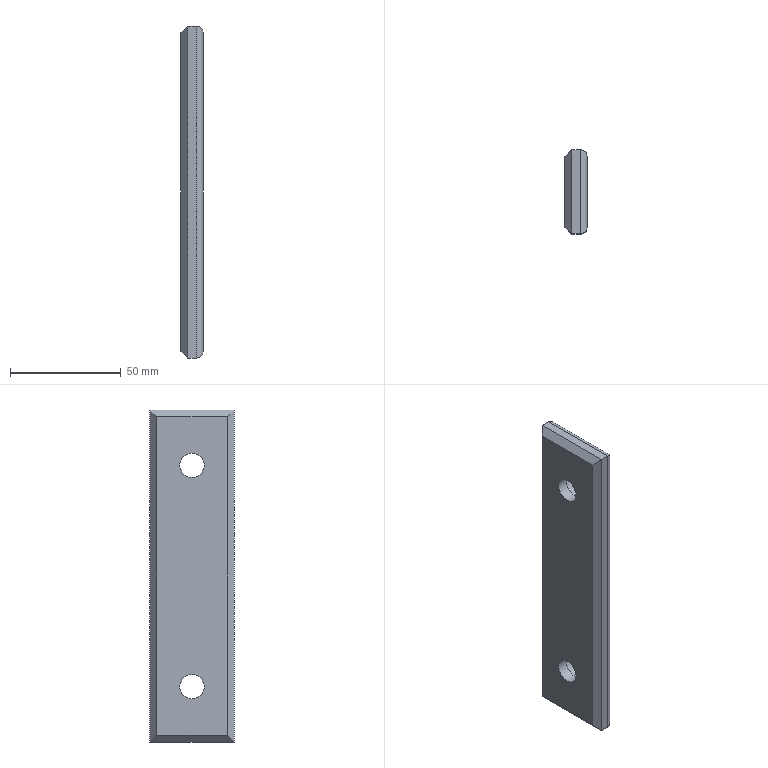Part | NX | features solid 2 | 1 solid | 20 faces | box 10 x 38 x 150 mm | volume 51273 mm3 | plane 12 | cylinder 8 | commonest cylinder face diameters 6 x4 11 x2 17.5 x2
STEP:
#1=CARTESIAN_POINT('',(163.,430.,45.));
#2=VERTEX_POINT('',#1);
#3=CARTESIAN_POINT('',(167.,430.,45.));
#4=VERTEX_POINT('',#3);
#5=CARTESIAN_POINT('',(160.,430.,45.));
#6=DIRECTION('',(1.,0.,0.));
#7=VECTOR('',#6,1000.);
#8=LINE('',#5,#7);
#9=EDGE_CURVE('',#2,#4,#8,.T.);
#10=ORIENTED_EDGE('',*,*,#9,.T.);
#11=CARTESIAN_POINT('',(167.,392.,45.));
#12=VERTEX_POINT('',#11);
#13=CARTESIAN_POINT('',(167.,392.,45.));
#14=DIRECTION('',(0.,1.,0.));
#15=VECTOR('',#14,1000.);
#16=LINE('',#13,#15);
#17=EDGE_CURVE('',#12,#4,#16,.T.);
#18=ORIENTED_EDGE('',*,*,#17,.F.);
#19=CARTESIAN_POINT('',(163.,392.,45.));
#20=VERTEX_POINT('',#19);
#21=CARTESIAN_POINT('',(160.,392.,45.));
#22=DIRECTION('',(1.,0.,0.));
#23=VECTOR('',#22,1000.);
#24=LINE('',#21,#23);
#25=EDGE_CURVE('',#20,#12,#24,.T.);
#26=ORIENTED_EDGE('',*,*,#25,.F.);
#27=CARTESIAN_POINT('',(163.,392.,45.));
#28=DIRECTION('',(0.,-1.,0.));
#29=VECTOR('',#28,1000.);
#30=LINE('',#27,#29);
#31=EDGE_CURVE('',#2,#20,#30,.T.);
#32=ORIENTED_EDGE('',*,*,#31,.F.);
#33=EDGE_LOOP('',(#10,#18,#26,#32));
#34=FACE_BOUND('',#33,.T.);
#35=CARTESIAN_POINT('',(160.,392.,45.));
#36=DIRECTION('',(0.,0.,1.));
#37=DIRECTION('',(1.,0.,0.));
#38=AXIS2_PLACEMENT_3D('',#35,#36,#37);
#39=PLANE('',#38);
#40=ADVANCED_FACE('',(#34),#39,.F.);
#41=CARTESIAN_POINT('',(163.,430.,195.));
#42=VERTEX_POINT('',#41);
#43=CARTESIAN_POINT('',(167.,430.,195.));
#44=VERTEX_POINT('',#43);
#45=CARTESIAN_POINT('',(160.,430.,195.));
#46=DIRECTION('',(1.,0.,0.));
#47=VECTOR('',#46,1000.);
#48=LINE('',#45,#47);
#49=EDGE_CURVE('',#42,#44,#48,.T.);
#50=ORIENTED_EDGE('',*,*,#49,.T.);
#51=CARTESIAN_POINT('',(167.,430.,45.));
#52=DIRECTION('',(0.,0.,1.));
#53=VECTOR('',#52,1000.);
#54=LINE('',#51,#53);
#55=EDGE_CURVE('',#4,#44,#54,.T.);
#56=ORIENTED_EDGE('',*,*,#55,.F.);
#57=ORIENTED_EDGE('',*,*,#9,.F.);
#58=CARTESIAN_POINT('',(163.,430.,45.));
#59=DIRECTION('',(0.,0.,-1.));
#60=VECTOR('',#59,1000.);
#61=LINE('',#58,#60);
#62=EDGE_CURVE('',#42,#2,#61,.T.);
#63=ORIENTED_EDGE('',*,*,#62,.F.);
#64=EDGE_LOOP('',(#50,#56,#57,#63));
#65=FACE_BOUND('',#64,.T.);
#66=CARTESIAN_POINT('',(160.,430.,45.));
#67=DIRECTION('',(0.,-1.,0.));
#68=DIRECTION('',(-1.,0.,0.));
#69=AXIS2_PLACEMENT_3D('',#66,#67,#68);
#70=PLANE('',#69);
#71=ADVANCED_FACE('',(#65),#70,.F.);
#72=CARTESIAN_POINT('',(163.,392.,195.));
#73=VERTEX_POINT('',#72);
#74=CARTESIAN_POINT('',(167.,392.,195.));
#75=VERTEX_POINT('',#74);
#76=CARTESIAN_POINT('',(160.,392.,195.));
#77=DIRECTION('',(1.,0.,0.));
#78=VECTOR('',#77,1000.);
#79=LINE('',#76,#78);
#80=EDGE_CURVE('',#73,#75,#79,.T.);
#81=ORIENTED_EDGE('',*,*,#80,.T.);
#82=CARTESIAN_POINT('',(167.,430.,195.));
#83=DIRECTION('',(0.,-1.,0.));
#84=VECTOR('',#83,1000.);
#85=LINE('',#82,#84);
#86=EDGE_CURVE('',#44,#75,#85,.T.);
#87=ORIENTED_EDGE('',*,*,#86,.F.);
#88=ORIENTED_EDGE('',*,*,#49,.F.);
#89=CARTESIAN_POINT('',(163.,430.,195.));
#90=DIRECTION('',(0.,1.,0.));
#91=VECTOR('',#90,1000.);
#92=LINE('',#89,#91);
#93=EDGE_CURVE('',#73,#42,#92,.T.);
#94=ORIENTED_EDGE('',*,*,#93,.F.);
#95=EDGE_LOOP('',(#81,#87,#88,#94));
#96=FACE_BOUND('',#95,.T.);
#97=CARTESIAN_POINT('',(160.,430.,195.));
#98=DIRECTION('',(0.,0.,-1.));
#99=DIRECTION('',(0.,1.,0.));
#100=AXIS2_PLACEMENT_3D('',#97,#98,#99);
#101=PLANE('',#100);
#102=ADVANCED_FACE('',(#96),#101,.F.);
#103=ORIENTED_EDGE('',*,*,#25,.T.);
#104=CARTESIAN_POINT('',(167.,392.,145.));
#105=DIRECTION('',(0.,0.,-1.));
#106=VECTOR('',#105,1000.);
#107=LINE('',#104,#106);
#108=EDGE_CURVE('',#75,#12,#107,.T.);
#109=ORIENTED_EDGE('',*,*,#108,.F.);
#110=ORIENTED_EDGE('',*,*,#80,.F.);
#111=CARTESIAN_POINT('',(163.,392.,145.));
#112=DIRECTION('',(0.,0.,1.));
#113=VECTOR('',#112,1000.);
#114=LINE('',#111,#113);
#115=EDGE_CURVE('',#20,#73,#114,.T.);
#116=ORIENTED_EDGE('',*,*,#115,.F.);
#117=EDGE_LOOP('',(#103,#109,#110,#116));
#118=FACE_BOUND('',#117,.T.);
#119=CARTESIAN_POINT('',(160.,392.,145.));
#120=DIRECTION('',(0.,1.,0.));
#121=DIRECTION('',(0.,0.,1.));
#122=AXIS2_PLACEMENT_3D('',#119,#120,#121);
#123=PLANE('',#122);
#124=ADVANCED_FACE('',(#118),#123,.F.);
#125=CARTESIAN_POINT('',(160.,427.,48.));
#126=VERTEX_POINT('',#125);
#127=CARTESIAN_POINT('',(160.,427.,192.));
#128=VERTEX_POINT('',#127);
#129=CARTESIAN_POINT('',(160.,427.,145.));
#130=DIRECTION('',(0.,0.,1.));
#131=VECTOR('',#130,1000.);
#132=LINE('',#129,#131);
#133=EDGE_CURVE('',#126,#128,#132,.T.);
#134=ORIENTED_EDGE('',*,*,#133,.F.);
#135=CARTESIAN_POINT('',(160.,395.,48.));
#136=VERTEX_POINT('',#135);
#137=CARTESIAN_POINT('',(160.,430.,48.));
#138=DIRECTION('',(0.,1.,0.));
#139=VECTOR('',#138,1000.);
#140=LINE('',#137,#139);
#141=EDGE_CURVE('',#136,#126,#140,.T.);
#142=ORIENTED_EDGE('',*,*,#141,.F.);
#143=CARTESIAN_POINT('',(160.,395.,192.));
#144=VERTEX_POINT('',#143);
#145=CARTESIAN_POINT('',(160.,395.,45.));
#146=DIRECTION('',(0.,0.,-1.));
#147=VECTOR('',#146,1000.);
#148=LINE('',#145,#147);
#149=EDGE_CURVE('',#144,#136,#148,.T.);
#150=ORIENTED_EDGE('',*,*,#149,.F.);
#151=CARTESIAN_POINT('',(160.,392.,192.));
#152=DIRECTION('',(0.,-1.,0.));
#153=VECTOR('',#152,1000.);
#154=LINE('',#151,#153);
#155=EDGE_CURVE('',#128,#144,#154,.T.);
#156=ORIENTED_EDGE('',*,*,#155,.F.);
#157=EDGE_LOOP('',(#134,#142,#150,#156));
#158=FACE_BOUND('',#157,.T.);
#159=CARTESIAN_POINT('',(160.,411.,175.5));
#160=VERTEX_POINT('',#159);
#161=CARTESIAN_POINT('',(160.,411.,170.));
#162=DIRECTION('',(1.,0.,0.));
#163=DIRECTION('',(0.,0.,1.));
#164=AXIS2_PLACEMENT_3D('',#161,#162,#163);
#165=CIRCLE('',#164,5.5);
#166=EDGE_CURVE('',#160,#160,#165,.T.);
#167=ORIENTED_EDGE('',*,*,#166,.T.);
#168=EDGE_LOOP('',(#167));
#169=FACE_BOUND('',#168,.T.);
#170=CARTESIAN_POINT('',(160.,411.,75.5));
#171=VERTEX_POINT('',#170);
#172=CARTESIAN_POINT('',(160.,411.,70.));
#173=DIRECTION('',(1.,0.,0.));
#174=DIRECTION('',(0.,0.,1.));
#175=AXIS2_PLACEMENT_3D('',#172,#173,#174);
#176=CIRCLE('',#175,5.5);
#177=EDGE_CURVE('',#171,#171,#176,.T.);
#178=ORIENTED_EDGE('',*,*,#177,.T.);
#179=EDGE_LOOP('',(#178));
#180=FACE_BOUND('',#179,.T.);
#181=CARTESIAN_POINT('',(160.,430.,45.));
#182=DIRECTION('',(-1.,0.,0.));
#183=DIRECTION('',(0.,0.,1.));
#184=AXIS2_PLACEMENT_3D('',#181,#182,#183);
#185=PLANE('',#184);
#186=ADVANCED_FACE('',(#158,#169,#180),#185,.T.);
#187=CARTESIAN_POINT('',(170.,427.,48.));
#188=VERTEX_POINT('',#187);
#189=CARTESIAN_POINT('',(170.,395.,48.));
#190=VERTEX_POINT('',#189);
#191=CARTESIAN_POINT('',(170.,430.,48.));
#192=DIRECTION('',(0.,1.,0.));
#193=VECTOR('',#192,1000.);
#194=LINE('',#191,#193);
#195=EDGE_CURVE('',#188,#190,#194,.F.);
#196=ORIENTED_EDGE('',*,*,#195,.F.);
#197=CARTESIAN_POINT('',(170.,427.,192.));
#198=VERTEX_POINT('',#197);
#199=CARTESIAN_POINT('',(170.,427.,45.));
#200=DIRECTION('',(0.,0.,1.));
#201=VECTOR('',#200,1000.);
#202=LINE('',#199,#201);
#203=EDGE_CURVE('',#198,#188,#202,.F.);
#204=ORIENTED_EDGE('',*,*,#203,.F.);
#205=CARTESIAN_POINT('',(170.,395.,192.));
#206=VERTEX_POINT('',#205);
#207=CARTESIAN_POINT('',(170.,430.,192.));
#208=DIRECTION('',(0.,-1.,0.));
#209=VECTOR('',#208,1000.);
#210=LINE('',#207,#209);
#211=EDGE_CURVE('',#206,#198,#210,.F.);
#212=ORIENTED_EDGE('',*,*,#211,.F.);
#213=CARTESIAN_POINT('',(170.,395.,45.));
#214=DIRECTION('',(0.,0.,-1.));
#215=VECTOR('',#214,1000.);
#216=LINE('',#213,#215);
#217=EDGE_CURVE('',#190,#206,#216,.F.);
#218=ORIENTED_EDGE('',*,*,#217,.F.);
#219=EDGE_LOOP('',(#196,#204,#212,#218));
#220=FACE_BOUND('',#219,.T.);
#221=CARTESIAN_POINT('',(170.,411.,178.75));
#222=VERTEX_POINT('',#221);
#223=CARTESIAN_POINT('',(170.,411.,170.));
#224=DIRECTION('',(1.,0.,0.));
#225=DIRECTION('',(0.,0.,1.));
#226=AXIS2_PLACEMENT_3D('',#223,#224,#225);
#227=CIRCLE('',#226,8.75);
#228=EDGE_CURVE('',#222,#222,#227,.T.);
#229=ORIENTED_EDGE('',*,*,#228,.F.);
#230=EDGE_LOOP('',(#229));
#231=FACE_BOUND('',#230,.T.);
#232=CARTESIAN_POINT('',(170.,411.,78.75));
#233=VERTEX_POINT('',#232);
#234=CARTESIAN_POINT('',(170.,411.,70.));
#235=DIRECTION('',(1.,0.,0.));
#236=DIRECTION('',(0.,0.,1.));
#237=AXIS2_PLACEMENT_3D('',#234,#235,#236);
#238=CIRCLE('',#237,8.75);
#239=EDGE_CURVE('',#233,#233,#238,.T.);
#240=ORIENTED_EDGE('',*,*,#239,.F.);
#241=EDGE_LOOP('',(#240));
#242=FACE_BOUND('',#241,.T.);
#243=CARTESIAN_POINT('',(170.,430.,45.));
#244=DIRECTION('',(-1.,0.,0.));
#245=DIRECTION('',(0.,0.,1.));
#246=AXIS2_PLACEMENT_3D('',#243,#244,#245);
#247=PLANE('',#246);
#248=ADVANCED_FACE('',(#220,#231,#242),#247,.F.);
#249=ORIENTED_EDGE('',*,*,#177,.F.);
#250=EDGE_LOOP('',(#249));
#251=FACE_BOUND('',#250,.T.);
#252=CARTESIAN_POINT('',(165.,411.,64.5));
#253=VERTEX_POINT('',#252);
#254=CARTESIAN_POINT('',(165.,411.,70.));
#255=DIRECTION('',(1.,0.,0.));
#256=DIRECTION('',(0.,0.,-1.));
#257=AXIS2_PLACEMENT_3D('',#254,#255,#256);
#258=CIRCLE('',#257,5.5);
#259=EDGE_CURVE('',#253,#253,#258,.T.);
#260=ORIENTED_EDGE('',*,*,#259,.T.);
#261=EDGE_LOOP('',(#260));
#262=FACE_BOUND('',#261,.T.);
#263=CARTESIAN_POINT('',(130.,411.,70.));
#264=DIRECTION('',(-1.,0.,0.));
#265=DIRECTION('',(0.,0.,1.));
#266=AXIS2_PLACEMENT_3D('',#263,#264,#265);
#267=CYLINDRICAL_SURFACE('',#266,5.5);
#268=ADVANCED_FACE('',(#251,#262),#267,.F.);
#269=ORIENTED_EDGE('',*,*,#259,.F.);
#270=EDGE_LOOP('',(#269));
#271=FACE_BOUND('',#270,.T.);
#272=CARTESIAN_POINT('',(165.,411.,61.25));
#273=VERTEX_POINT('',#272);
#274=CARTESIAN_POINT('',(165.,411.,70.));
#275=DIRECTION('',(1.,0.,0.));
#276=DIRECTION('',(0.,0.,-1.));
#277=AXIS2_PLACEMENT_3D('',#274,#275,#276);
#278=CIRCLE('',#277,8.75);
#279=EDGE_CURVE('',#273,#273,#278,.T.);
#280=ORIENTED_EDGE('',*,*,#279,.T.);
#281=EDGE_LOOP('',(#280));
#282=FACE_BOUND('',#281,.T.);
#283=CARTESIAN_POINT('',(165.,411.,70.));
#284=DIRECTION('',(-1.,0.,0.));
#285=DIRECTION('',(0.,0.,1.));
#286=AXIS2_PLACEMENT_3D('',#283,#284,#285);
#287=PLANE('',#286);
#288=ADVANCED_FACE('',(#271,#282),#287,.F.);
#289=ORIENTED_EDGE('',*,*,#279,.F.);
#290=EDGE_LOOP('',(#289));
#291=FACE_BOUND('',#290,.T.);
#292=ORIENTED_EDGE('',*,*,#239,.T.);
#293=EDGE_LOOP('',(#292));
#294=FACE_BOUND('',#293,.T.);
#295=CARTESIAN_POINT('',(180.,411.,70.));
#296=DIRECTION('',(-1.,0.,0.));
#297=DIRECTION('',(0.,0.,1.));
#298=AXIS2_PLACEMENT_3D('',#295,#296,#297);
#299=CYLINDRICAL_SURFACE('',#298,8.75);
#300=ADVANCED_FACE('',(#291,#294),#299,.F.);
#301=ORIENTED_EDGE('',*,*,#166,.F.);
#302=EDGE_LOOP('',(#301));
#303=FACE_BOUND('',#302,.T.);
#304=CARTESIAN_POINT('',(165.,411.,164.5));
#305=VERTEX_POINT('',#304);
#306=CARTESIAN_POINT('',(165.,411.,170.));
#307=DIRECTION('',(1.,0.,0.));
#308=DIRECTION('',(0.,0.,-1.));
#309=AXIS2_PLACEMENT_3D('',#306,#307,#308);
#310=CIRCLE('',#309,5.5);
#311=EDGE_CURVE('',#305,#305,#310,.T.);
#312=ORIENTED_EDGE('',*,*,#311,.T.);
#313=EDGE_LOOP('',(#312));
#314=FACE_BOUND('',#313,.T.);
#315=CARTESIAN_POINT('',(130.,411.,170.));
#316=DIRECTION('',(-1.,0.,0.));
#317=DIRECTION('',(0.,0.,1.));
#318=AXIS2_PLACEMENT_3D('',#315,#316,#317);
#319=CYLINDRICAL_SURFACE('',#318,5.5);
#320=ADVANCED_FACE('',(#303,#314),#319,.F.);
#321=ORIENTED_EDGE('',*,*,#311,.F.);
#322=EDGE_LOOP('',(#321));
#323=FACE_BOUND('',#322,.T.);
#324=CARTESIAN_POINT('',(165.,411.,161.25));
#325=VERTEX_POINT('',#324);
#326=CARTESIAN_POINT('',(165.,411.,170.));
#327=DIRECTION('',(1.,0.,0.));
#328=DIRECTION('',(0.,0.,-1.));
#329=AXIS2_PLACEMENT_3D('',#326,#327,#328);
#330=CIRCLE('',#329,8.75);
#331=EDGE_CURVE('',#325,#325,#330,.T.);
#332=ORIENTED_EDGE('',*,*,#331,.T.);
#333=EDGE_LOOP('',(#332));
#334=FACE_BOUND('',#333,.T.);
#335=CARTESIAN_POINT('',(165.,411.,120.));
#336=DIRECTION('',(-1.,0.,0.));
#337=DIRECTION('',(0.,0.,1.));
#338=AXIS2_PLACEMENT_3D('',#335,#336,#337);
#339=PLANE('',#338);
#340=ADVANCED_FACE('',(#323,#334),#339,.F.);
#341=ORIENTED_EDGE('',*,*,#331,.F.);
#342=EDGE_LOOP('',(#341));
#343=FACE_BOUND('',#342,.T.);
#344=ORIENTED_EDGE('',*,*,#228,.T.);
#345=EDGE_LOOP('',(#344));
#346=FACE_BOUND('',#345,.T.);
#347=CARTESIAN_POINT('',(180.,411.,170.));
#348=DIRECTION('',(-1.,0.,0.));
#349=DIRECTION('',(0.,0.,1.));
#350=AXIS2_PLACEMENT_3D('',#347,#348,#349);
#351=CYLINDRICAL_SURFACE('',#350,8.75);
#352=ADVANCED_FACE('',(#343,#346),#351,.F.);
#353=CARTESIAN_POINT('',(167.,427.,48.));
#354=DIRECTION('',(0.,-0.7071,-0.7071));
#355=DIRECTION('',(0.,0.7071,-0.7071));
#356=AXIS2_PLACEMENT_3D('',#353,#354,#355);
#357=ELLIPSE('',#356,4.243,3.);
#358=EDGE_CURVE('',#188,#4,#357,.F.);
#359=ORIENTED_EDGE('',*,*,#358,.T.);
#360=ORIENTED_EDGE('',*,*,#55,.T.);
#361=CARTESIAN_POINT('',(167.,427.,192.));
#362=DIRECTION('',(0.,0.7071,-0.7071));
#363=DIRECTION('',(0.,0.7071,0.7071));
#364=AXIS2_PLACEMENT_3D('',#361,#362,#363);
#365=ELLIPSE('',#364,4.243,3.);
#366=EDGE_CURVE('',#44,#198,#365,.T.);
#367=ORIENTED_EDGE('',*,*,#366,.T.);
#368=ORIENTED_EDGE('',*,*,#203,.T.);
#369=EDGE_LOOP('',(#359,#360,#367,#368));
#370=FACE_BOUND('',#369,.T.);
#371=CARTESIAN_POINT('',(167.,427.,45.));
#372=DIRECTION('',(0.,0.,1.));
#373=DIRECTION('',(1.,0.,0.));
#374=AXIS2_PLACEMENT_3D('',#371,#372,#373);
#375=CYLINDRICAL_SURFACE('',#374,3.);
#376=ADVANCED_FACE('',(#370),#375,.T.);
#377=ORIENTED_EDGE('',*,*,#366,.F.);
#378=ORIENTED_EDGE('',*,*,#86,.T.);
#379=CARTESIAN_POINT('',(167.,395.,192.));
#380=DIRECTION('',(0.,0.7071,0.7071));
#381=DIRECTION('',(0.,-0.7071,0.7071));
#382=AXIS2_PLACEMENT_3D('',#379,#380,#381);
#383=ELLIPSE('',#382,4.243,3.);
#384=EDGE_CURVE('',#75,#206,#383,.T.);
#385=ORIENTED_EDGE('',*,*,#384,.T.);
#386=ORIENTED_EDGE('',*,*,#211,.T.);
#387=EDGE_LOOP('',(#377,#378,#385,#386));
#388=FACE_BOUND('',#387,.T.);
#389=CARTESIAN_POINT('',(167.,430.,192.));
#390=DIRECTION('',(0.,-1.,0.));
#391=DIRECTION('',(0.,0.,-1.));
#392=AXIS2_PLACEMENT_3D('',#389,#390,#391);
#393=CYLINDRICAL_SURFACE('',#392,3.);
#394=ADVANCED_FACE('',(#388),#393,.T.);
#395=ORIENTED_EDGE('',*,*,#358,.F.);
#396=ORIENTED_EDGE('',*,*,#195,.T.);
#397=CARTESIAN_POINT('',(167.,395.,48.));
#398=DIRECTION('',(0.,-0.7071,0.7071));
#399=DIRECTION('',(0.,0.7071,0.7071));
#400=AXIS2_PLACEMENT_3D('',#397,#398,#399);
#401=ELLIPSE('',#400,4.243,3.);
#402=EDGE_CURVE('',#190,#12,#401,.F.);
#403=ORIENTED_EDGE('',*,*,#402,.T.);
#404=ORIENTED_EDGE('',*,*,#17,.T.);
#405=EDGE_LOOP('',(#395,#396,#403,#404));
#406=FACE_BOUND('',#405,.T.);
#407=CARTESIAN_POINT('',(167.,392.,48.));
#408=DIRECTION('',(0.,1.,0.));
#409=DIRECTION('',(1.,0.,0.));
#410=AXIS2_PLACEMENT_3D('',#407,#408,#409);
#411=CYLINDRICAL_SURFACE('',#410,3.);
#412=ADVANCED_FACE('',(#406),#411,.T.);
#413=ORIENTED_EDGE('',*,*,#384,.F.);
#414=ORIENTED_EDGE('',*,*,#108,.T.);
#415=ORIENTED_EDGE('',*,*,#402,.F.);
#416=ORIENTED_EDGE('',*,*,#217,.T.);
#417=EDGE_LOOP('',(#413,#414,#415,#416));
#418=FACE_BOUND('',#417,.T.);
#419=CARTESIAN_POINT('',(167.,395.,145.));
#420=DIRECTION('',(0.,0.,-1.));
#421=DIRECTION('',(0.,1.,0.));
#422=AXIS2_PLACEMENT_3D('',#419,#420,#421);
#423=CYLINDRICAL_SURFACE('',#422,3.);
#424=ADVANCED_FACE('',(#418),#423,.T.);
#425=CARTESIAN_POINT('',(161.,394.,47.));
#426=DIRECTION('',(-0.5774,0.5774,0.5774));
#427=VECTOR('',#426,1000.);
#428=LINE('',#425,#427);
#429=EDGE_CURVE('',#20,#136,#428,.T.);
#430=ORIENTED_EDGE('',*,*,#429,.T.);
#431=ORIENTED_EDGE('',*,*,#141,.T.);
#432=CARTESIAN_POINT('',(161.,428.,47.));
#433=DIRECTION('',(-0.5774,-0.5774,0.5774));
#434=VECTOR('',#433,1000.);
#435=LINE('',#432,#434);
#436=EDGE_CURVE('',#126,#2,#435,.F.);
#437=ORIENTED_EDGE('',*,*,#436,.T.);
#438=ORIENTED_EDGE('',*,*,#31,.T.);
#439=EDGE_LOOP('',(#430,#431,#437,#438));
#440=FACE_BOUND('',#439,.T.);
#441=CARTESIAN_POINT('',(160.,430.,48.));
#442=DIRECTION('',(-0.7071,0.,-0.7071));
#443=DIRECTION('',(-0.7071,0.,0.7071));
#444=AXIS2_PLACEMENT_3D('',#441,#442,#443);
#445=PLANE('',#444);
#446=ADVANCED_FACE('',(#440),#445,.T.);
#447=ORIENTED_EDGE('',*,*,#436,.F.);
#448=ORIENTED_EDGE('',*,*,#133,.T.);
#449=CARTESIAN_POINT('',(127.667,394.667,159.667));
#450=DIRECTION('',(-0.5774,-0.5774,-0.5774));
#451=VECTOR('',#450,1000.);
#452=LINE('',#449,#451);
#453=EDGE_CURVE('',#128,#42,#452,.F.);
#454=ORIENTED_EDGE('',*,*,#453,.T.);
#455=ORIENTED_EDGE('',*,*,#62,.T.);
#456=EDGE_LOOP('',(#447,#448,#454,#455));
#457=FACE_BOUND('',#456,.T.);
#458=CARTESIAN_POINT('',(160.,427.,45.));
#459=DIRECTION('',(-0.7071,0.7071,0.));
#460=DIRECTION('',(0.7071,0.7071,0.));
#461=AXIS2_PLACEMENT_3D('',#458,#459,#460);
#462=PLANE('',#461);
#463=ADVANCED_FACE('',(#457),#462,.T.);
#464=ORIENTED_EDGE('',*,*,#429,.F.);
#465=ORIENTED_EDGE('',*,*,#115,.T.);
#466=CARTESIAN_POINT('',(127.667,427.333,159.667));
#467=DIRECTION('',(0.5774,-0.5774,0.5774));
#468=VECTOR('',#467,1000.);
#469=LINE('',#466,#468);
#470=EDGE_CURVE('',#73,#144,#469,.F.);
#471=ORIENTED_EDGE('',*,*,#470,.T.);
#472=ORIENTED_EDGE('',*,*,#149,.T.);
#473=EDGE_LOOP('',(#464,#465,#471,#472));
#474=FACE_BOUND('',#473,.T.);
#475=CARTESIAN_POINT('',(160.,395.,45.));
#476=DIRECTION('',(-0.7071,-0.7071,0.));
#477=DIRECTION('',(-0.7071,0.7071,0.));
#478=AXIS2_PLACEMENT_3D('',#475,#476,#477);
#479=PLANE('',#478);
#480=ADVANCED_FACE('',(#474),#479,.T.);
#481=ORIENTED_EDGE('',*,*,#453,.F.);
#482=ORIENTED_EDGE('',*,*,#155,.T.);
#483=ORIENTED_EDGE('',*,*,#470,.F.);
#484=ORIENTED_EDGE('',*,*,#93,.T.);
#485=EDGE_LOOP('',(#481,#482,#483,#484));
#486=FACE_BOUND('',#485,.T.);
#487=CARTESIAN_POINT('',(160.,430.,192.));
#488=DIRECTION('',(-0.7071,0.,0.7071));
#489=DIRECTION('',(0.7071,0.,0.7071));
#490=AXIS2_PLACEMENT_3D('',#487,#488,#489);
#491=PLANE('',#490);
#492=ADVANCED_FACE('',(#486),#491,.T.);
#493=CLOSED_SHELL('',(#40,#71,#102,#124,#186,#248,#268,#288,#300,#320,#340,#352,#376,#394,#412,#424,#446,#463,#480,#492));
#494=MANIFOLD_SOLID_BREP('',#493);
#495=(LENGTH_UNIT()NAMED_UNIT(*)SI_UNIT(.MILLI.,.METRE.));
#496=UNCERTAINTY_MEASURE_WITH_UNIT(LENGTH_MEASURE(0.00001),#495,'','');
#497=(NAMED_UNIT(*)PLANE_ANGLE_UNIT()SI_UNIT($,.RADIAN.));
#498=(NAMED_UNIT(*)SI_UNIT($,.STERADIAN.)SOLID_ANGLE_UNIT());
#499=(GEOMETRIC_REPRESENTATION_CONTEXT(3)GLOBAL_UNCERTAINTY_ASSIGNED_CONTEXT((#496))GLOBAL_UNIT_ASSIGNED_CONTEXT((#495,#497,#498))REPRESENTATION_CONTEXT('',''));
#500=ADVANCED_BREP_SHAPE_REPRESENTATION('',(#494),#499);